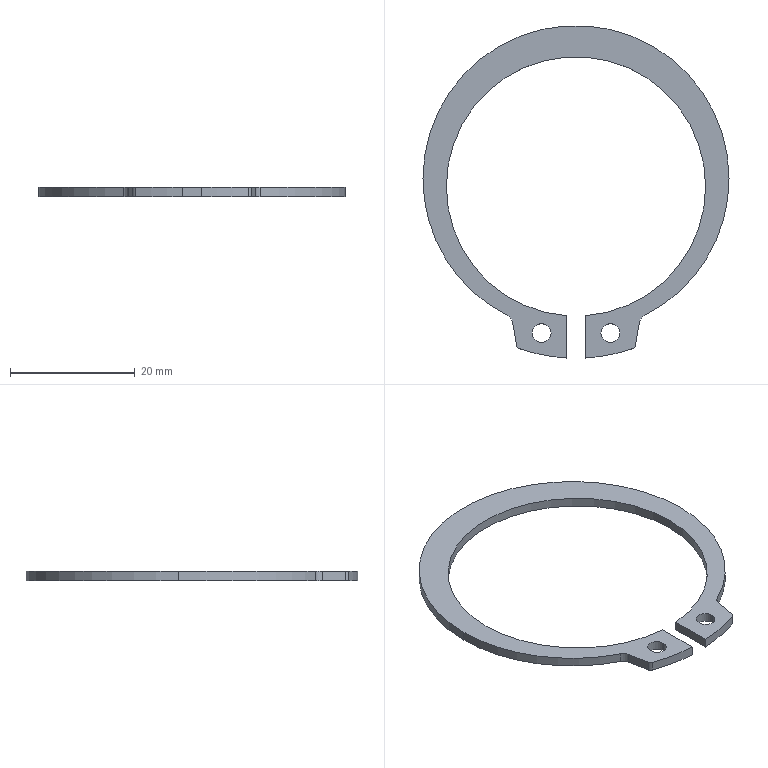Part | SolidWorks | features Extrusion 1 | 1 solid | 22 faces | box 49 x 53.209 x 1.5 mm | volume 876.142 mm3 | cylinder 16 | plane 6 | commonest cylinder face diameters 3 x6 41.5 x3 49 x3 1.4 x2 55 x2
STEP:
#1=CARTESIAN_POINT('',(4.,-24.714,0.75));
#2=VERTEX_POINT('',#1);
#3=CARTESIAN_POINT('',(7.,-24.714,0.75));
#4=VERTEX_POINT('',#3);
#5=CARTESIAN_POINT('',(5.5,-24.714,0.75));
#6=DIRECTION('',(0.,0.,1.));
#7=DIRECTION('',(-1.,0.,0.));
#8=AXIS2_PLACEMENT_3D('',#5,#6,#7);
#9=CIRCLE('',#8,1.5);
#10=EDGE_CURVE('',#2,#4,#9,.T.);
#11=ORIENTED_EDGE('',*,*,#10,.T.);
#12=CARTESIAN_POINT('',(7.,-24.714,-0.75));
#13=VERTEX_POINT('',#12);
#14=CARTESIAN_POINT('',(7.,-24.714,0.75));
#15=DIRECTION('',(0.,0.,-1.));
#16=VECTOR('',#15,1000.);
#17=LINE('',#14,#16);
#18=EDGE_CURVE('',#4,#13,#17,.T.);
#19=ORIENTED_EDGE('',*,*,#18,.T.);
#20=CARTESIAN_POINT('',(4.,-24.714,-0.75));
#21=VERTEX_POINT('',#20);
#22=CARTESIAN_POINT('',(5.5,-24.714,-0.75));
#23=DIRECTION('',(0.,0.,1.));
#24=DIRECTION('',(-1.,0.,0.));
#25=AXIS2_PLACEMENT_3D('',#22,#23,#24);
#26=CIRCLE('',#25,1.5);
#27=EDGE_CURVE('',#21,#13,#26,.T.);
#28=ORIENTED_EDGE('',*,*,#27,.F.);
#29=CARTESIAN_POINT('',(4.,-24.714,0.75));
#30=DIRECTION('',(0.,0.,-1.));
#31=VECTOR('',#30,1000.);
#32=LINE('',#29,#31);
#33=EDGE_CURVE('',#2,#21,#32,.T.);
#34=ORIENTED_EDGE('',*,*,#33,.F.);
#35=EDGE_LOOP('',(#11,#19,#28,#34));
#36=FACE_OUTER_BOUND('',#35,.T.);
#37=CARTESIAN_POINT('',(5.5,-24.714,0.75));
#38=DIRECTION('',(0.,0.,-1.));
#39=DIRECTION('',(-1.,0.,0.));
#40=AXIS2_PLACEMENT_3D('',#37,#38,#39);
#41=CYLINDRICAL_SURFACE('',#40,1.5);
#42=ADVANCED_FACE('',(#36),#41,.F.);
#43=CARTESIAN_POINT('',(-7.,-24.714,0.75));
#44=VERTEX_POINT('',#43);
#45=CARTESIAN_POINT('',(-4.,-24.714,0.75));
#46=VERTEX_POINT('',#45);
#47=CARTESIAN_POINT('',(-5.5,-24.714,0.75));
#48=DIRECTION('',(0.,0.,1.));
#49=DIRECTION('',(1.,0.,0.));
#50=AXIS2_PLACEMENT_3D('',#47,#48,#49);
#51=CIRCLE('',#50,1.5);
#52=EDGE_CURVE('',#44,#46,#51,.T.);
#53=ORIENTED_EDGE('',*,*,#52,.T.);
#54=CARTESIAN_POINT('',(-4.,-24.714,-0.75));
#55=VERTEX_POINT('',#54);
#56=CARTESIAN_POINT('',(-4.,-24.714,0.75));
#57=DIRECTION('',(0.,0.,-1.));
#58=VECTOR('',#57,1000.);
#59=LINE('',#56,#58);
#60=EDGE_CURVE('',#46,#55,#59,.T.);
#61=ORIENTED_EDGE('',*,*,#60,.T.);
#62=CARTESIAN_POINT('',(-7.,-24.714,-0.75));
#63=VERTEX_POINT('',#62);
#64=CARTESIAN_POINT('',(-5.5,-24.714,-0.75));
#65=DIRECTION('',(0.,0.,1.));
#66=DIRECTION('',(1.,0.,0.));
#67=AXIS2_PLACEMENT_3D('',#64,#65,#66);
#68=CIRCLE('',#67,1.5);
#69=EDGE_CURVE('',#63,#55,#68,.T.);
#70=ORIENTED_EDGE('',*,*,#69,.F.);
#71=CARTESIAN_POINT('',(-7.,-24.714,0.75));
#72=DIRECTION('',(0.,0.,-1.));
#73=VECTOR('',#72,1000.);
#74=LINE('',#71,#73);
#75=EDGE_CURVE('',#44,#63,#74,.T.);
#76=ORIENTED_EDGE('',*,*,#75,.F.);
#77=EDGE_LOOP('',(#53,#61,#70,#76));
#78=FACE_OUTER_BOUND('',#77,.T.);
#79=CARTESIAN_POINT('',(-5.5,-24.714,0.75));
#80=DIRECTION('',(0.,0.,-1.));
#81=DIRECTION('',(-1.,0.,0.));
#82=AXIS2_PLACEMENT_3D('',#79,#80,#81);
#83=CYLINDRICAL_SURFACE('',#82,1.5);
#84=ADVANCED_FACE('',(#78),#83,.F.);
#85=CARTESIAN_POINT('',(24.5,0.,0.75));
#86=VERTEX_POINT('',#85);
#87=CARTESIAN_POINT('',(-24.5,0.,0.75));
#88=VERTEX_POINT('',#87);
#89=CARTESIAN_POINT('',(0.,0.,0.75));
#90=DIRECTION('',(0.,0.,1.));
#91=DIRECTION('',(1.,0.,0.));
#92=AXIS2_PLACEMENT_3D('',#89,#90,#91);
#93=CIRCLE('',#92,24.5);
#94=EDGE_CURVE('',#86,#88,#93,.T.);
#95=ORIENTED_EDGE('',*,*,#94,.F.);
#96=CARTESIAN_POINT('',(24.5,0.,-0.75));
#97=VERTEX_POINT('',#96);
#98=CARTESIAN_POINT('',(24.5,0.,0.75));
#99=DIRECTION('',(0.,0.,-1.));
#100=VECTOR('',#99,1000.);
#101=LINE('',#98,#100);
#102=EDGE_CURVE('',#86,#97,#101,.T.);
#103=ORIENTED_EDGE('',*,*,#102,.T.);
#104=CARTESIAN_POINT('',(-24.5,0.,-0.75));
#105=VERTEX_POINT('',#104);
#106=CARTESIAN_POINT('',(0.,0.,-0.75));
#107=DIRECTION('',(0.,0.,1.));
#108=DIRECTION('',(1.,0.,0.));
#109=AXIS2_PLACEMENT_3D('',#106,#107,#108);
#110=CIRCLE('',#109,24.5);
#111=EDGE_CURVE('',#97,#105,#110,.T.);
#112=ORIENTED_EDGE('',*,*,#111,.T.);
#113=CARTESIAN_POINT('',(-24.5,0.,0.75));
#114=DIRECTION('',(0.,0.,-1.));
#115=VECTOR('',#114,1000.);
#116=LINE('',#113,#115);
#117=EDGE_CURVE('',#88,#105,#116,.T.);
#118=ORIENTED_EDGE('',*,*,#117,.F.);
#119=EDGE_LOOP('',(#95,#103,#112,#118));
#120=FACE_OUTER_BOUND('',#119,.T.);
#121=CARTESIAN_POINT('',(0.,0.,0.75));
#122=DIRECTION('',(0.,0.,-1.));
#123=DIRECTION('',(-1.,0.,0.));
#124=AXIS2_PLACEMENT_3D('',#121,#122,#123);
#125=CYLINDRICAL_SURFACE('',#124,24.5);
#126=ADVANCED_FACE('',(#120),#125,.T.);
#127=CARTESIAN_POINT('',(-10.957,-21.914,0.75));
#128=VERTEX_POINT('',#127);
#129=CARTESIAN_POINT('',(0.,0.,0.75));
#130=DIRECTION('',(0.,0.,1.));
#131=DIRECTION('',(1.,0.,0.));
#132=AXIS2_PLACEMENT_3D('',#129,#130,#131);
#133=CIRCLE('',#132,24.5);
#134=EDGE_CURVE('',#88,#128,#133,.T.);
#135=ORIENTED_EDGE('',*,*,#134,.F.);
#136=ORIENTED_EDGE('',*,*,#117,.T.);
#137=CARTESIAN_POINT('',(-10.957,-21.914,-0.75));
#138=VERTEX_POINT('',#137);
#139=CARTESIAN_POINT('',(0.,0.,-0.75));
#140=DIRECTION('',(0.,0.,1.));
#141=DIRECTION('',(1.,0.,0.));
#142=AXIS2_PLACEMENT_3D('',#139,#140,#141);
#143=CIRCLE('',#142,24.5);
#144=EDGE_CURVE('',#105,#138,#143,.T.);
#145=ORIENTED_EDGE('',*,*,#144,.T.);
#146=CARTESIAN_POINT('',(-10.957,-21.914,0.75));
#147=DIRECTION('',(0.,0.,-1.));
#148=VECTOR('',#147,1000.);
#149=LINE('',#146,#148);
#150=EDGE_CURVE('',#128,#138,#149,.T.);
#151=ORIENTED_EDGE('',*,*,#150,.F.);
#152=EDGE_LOOP('',(#135,#136,#145,#151));
#153=FACE_OUTER_BOUND('',#152,.T.);
#154=CARTESIAN_POINT('',(0.,0.,0.75));
#155=DIRECTION('',(0.,0.,-1.));
#156=DIRECTION('',(-1.,0.,0.));
#157=AXIS2_PLACEMENT_3D('',#154,#155,#156);
#158=CYLINDRICAL_SURFACE('',#157,24.5);
#159=ADVANCED_FACE('',(#153),#158,.T.);
#160=CARTESIAN_POINT('',(20.75,-1.25,0.75));
#161=VERTEX_POINT('',#160);
#162=CARTESIAN_POINT('',(1.5,-21.946,0.75));
#163=VERTEX_POINT('',#162);
#164=CARTESIAN_POINT('',(0.,-1.25,0.75));
#165=DIRECTION('',(0.,0.,-1.));
#166=DIRECTION('',(1.,0.,0.));
#167=AXIS2_PLACEMENT_3D('',#164,#165,#166);
#168=CIRCLE('',#167,20.75);
#169=EDGE_CURVE('',#161,#163,#168,.T.);
#170=ORIENTED_EDGE('',*,*,#169,.F.);
#171=CARTESIAN_POINT('',(20.75,-1.25,-0.75));
#172=VERTEX_POINT('',#171);
#173=CARTESIAN_POINT('',(20.75,-1.25,0.75));
#174=DIRECTION('',(0.,0.,-1.));
#175=VECTOR('',#174,1000.);
#176=LINE('',#173,#175);
#177=EDGE_CURVE('',#161,#172,#176,.T.);
#178=ORIENTED_EDGE('',*,*,#177,.T.);
#179=CARTESIAN_POINT('',(1.5,-21.946,-0.75));
#180=VERTEX_POINT('',#179);
#181=CARTESIAN_POINT('',(0.,-1.25,-0.75));
#182=DIRECTION('',(0.,0.,-1.));
#183=DIRECTION('',(1.,0.,0.));
#184=AXIS2_PLACEMENT_3D('',#181,#182,#183);
#185=CIRCLE('',#184,20.75);
#186=EDGE_CURVE('',#172,#180,#185,.T.);
#187=ORIENTED_EDGE('',*,*,#186,.T.);
#188=CARTESIAN_POINT('',(1.5,-21.946,0.75));
#189=DIRECTION('',(0.,0.,-1.));
#190=VECTOR('',#189,1000.);
#191=LINE('',#188,#190);
#192=EDGE_CURVE('',#163,#180,#191,.T.);
#193=ORIENTED_EDGE('',*,*,#192,.F.);
#194=EDGE_LOOP('',(#170,#178,#187,#193));
#195=FACE_OUTER_BOUND('',#194,.T.);
#196=CARTESIAN_POINT('',(0.,-1.25,0.75));
#197=DIRECTION('',(0.,0.,-1.));
#198=DIRECTION('',(-1.,0.,0.));
#199=AXIS2_PLACEMENT_3D('',#196,#197,#198);
#200=CYLINDRICAL_SURFACE('',#199,20.75);
#201=ADVANCED_FACE('',(#195),#200,.F.);
#202=ORIENTED_EDGE('',*,*,#177,.F.);
#203=CARTESIAN_POINT('',(-20.75,-1.25,0.75));
#204=VERTEX_POINT('',#203);
#205=CARTESIAN_POINT('',(0.,-1.25,0.75));
#206=DIRECTION('',(0.,0.,-1.));
#207=DIRECTION('',(1.,0.,0.));
#208=AXIS2_PLACEMENT_3D('',#205,#206,#207);
#209=CIRCLE('',#208,20.75);
#210=EDGE_CURVE('',#204,#161,#209,.T.);
#211=ORIENTED_EDGE('',*,*,#210,.F.);
#212=CARTESIAN_POINT('',(-20.75,-1.25,-0.75));
#213=VERTEX_POINT('',#212);
#214=CARTESIAN_POINT('',(-20.75,-1.25,0.75));
#215=DIRECTION('',(0.,0.,-1.));
#216=VECTOR('',#215,1000.);
#217=LINE('',#214,#216);
#218=EDGE_CURVE('',#204,#213,#217,.T.);
#219=ORIENTED_EDGE('',*,*,#218,.T.);
#220=CARTESIAN_POINT('',(0.,-1.25,-0.75));
#221=DIRECTION('',(0.,0.,-1.));
#222=DIRECTION('',(1.,0.,0.));
#223=AXIS2_PLACEMENT_3D('',#220,#221,#222);
#224=CIRCLE('',#223,20.75);
#225=EDGE_CURVE('',#213,#172,#224,.T.);
#226=ORIENTED_EDGE('',*,*,#225,.T.);
#227=EDGE_LOOP('',(#202,#211,#219,#226));
#228=FACE_OUTER_BOUND('',#227,.T.);
#229=CARTESIAN_POINT('',(0.,-1.25,0.75));
#230=DIRECTION('',(0.,0.,-1.));
#231=DIRECTION('',(-1.,0.,0.));
#232=AXIS2_PLACEMENT_3D('',#229,#230,#231);
#233=CYLINDRICAL_SURFACE('',#232,20.75);
#234=ADVANCED_FACE('',(#228),#233,.F.);
#235=ORIENTED_EDGE('',*,*,#52,.F.);
#236=CARTESIAN_POINT('',(-5.5,-24.714,0.75));
#237=DIRECTION('',(0.,0.,1.));
#238=DIRECTION('',(1.,0.,0.));
#239=AXIS2_PLACEMENT_3D('',#236,#237,#238);
#240=CIRCLE('',#239,1.5);
#241=EDGE_CURVE('',#46,#44,#240,.T.);
#242=ORIENTED_EDGE('',*,*,#241,.F.);
#243=EDGE_LOOP('',(#235,#242));
#244=FACE_BOUND('',#243,.T.);
#245=CARTESIAN_POINT('',(-10.15,-22.995,0.75));
#246=VERTEX_POINT('',#245);
#247=CARTESIAN_POINT('',(-11.627,-23.255,0.75));
#248=DIRECTION('',(0.,0.,-1.));
#249=DIRECTION('',(1.,0.,0.));
#250=AXIS2_PLACEMENT_3D('',#247,#248,#249);
#251=CIRCLE('',#250,1.5);
#252=EDGE_CURVE('',#128,#246,#251,.T.);
#253=ORIENTED_EDGE('',*,*,#252,.T.);
#254=CARTESIAN_POINT('',(-9.5,-26.682,0.75));
#255=VERTEX_POINT('',#254);
#256=CARTESIAN_POINT('',(-10.15,-22.995,0.75));
#257=DIRECTION('',(0.1736,-0.9848,0.));
#258=VECTOR('',#257,1000.);
#259=LINE('',#256,#258);
#260=EDGE_CURVE('',#246,#255,#259,.T.);
#261=ORIENTED_EDGE('',*,*,#260,.T.);
#262=CARTESIAN_POINT('',(-9.041,-27.221,0.75));
#263=VERTEX_POINT('',#262);
#264=CARTESIAN_POINT('',(-8.811,-26.56,0.75));
#265=DIRECTION('',(0.,0.,1.));
#266=DIRECTION('',(-1.,0.,0.));
#267=AXIS2_PLACEMENT_3D('',#264,#265,#266);
#268=CIRCLE('',#267,0.7);
#269=EDGE_CURVE('',#255,#263,#268,.T.);
#270=ORIENTED_EDGE('',*,*,#269,.T.);
#271=CARTESIAN_POINT('',(-1.5,-28.709,0.75));
#272=VERTEX_POINT('',#271);
#273=CARTESIAN_POINT('',(0.,-1.25,0.75));
#274=DIRECTION('',(0.,0.,1.));
#275=DIRECTION('',(-1.,0.,0.));
#276=AXIS2_PLACEMENT_3D('',#273,#274,#275);
#277=CIRCLE('',#276,27.5);
#278=EDGE_CURVE('',#263,#272,#277,.T.);
#279=ORIENTED_EDGE('',*,*,#278,.T.);
#280=CARTESIAN_POINT('',(-1.5,-21.946,0.75));
#281=VERTEX_POINT('',#280);
#282=CARTESIAN_POINT('',(-1.5,-21.946,0.75));
#283=DIRECTION('',(0.,1.,0.));
#284=VECTOR('',#283,1000.);
#285=LINE('',#282,#284);
#286=EDGE_CURVE('',#272,#281,#285,.T.);
#287=ORIENTED_EDGE('',*,*,#286,.T.);
#288=CARTESIAN_POINT('',(0.,-1.25,0.75));
#289=DIRECTION('',(0.,0.,-1.));
#290=DIRECTION('',(1.,0.,0.));
#291=AXIS2_PLACEMENT_3D('',#288,#289,#290);
#292=CIRCLE('',#291,20.75);
#293=EDGE_CURVE('',#281,#204,#292,.T.);
#294=ORIENTED_EDGE('',*,*,#293,.T.);
#295=ORIENTED_EDGE('',*,*,#210,.T.);
#296=ORIENTED_EDGE('',*,*,#169,.T.);
#297=CARTESIAN_POINT('',(1.5,-28.709,0.75));
#298=VERTEX_POINT('',#297);
#299=CARTESIAN_POINT('',(1.5,-21.946,0.75));
#300=DIRECTION('',(0.,-1.,0.));
#301=VECTOR('',#300,1000.);
#302=LINE('',#299,#301);
#303=EDGE_CURVE('',#163,#298,#302,.T.);
#304=ORIENTED_EDGE('',*,*,#303,.T.);
#305=CARTESIAN_POINT('',(9.041,-27.221,0.75));
#306=VERTEX_POINT('',#305);
#307=CARTESIAN_POINT('',(0.,-1.25,0.75));
#308=DIRECTION('',(0.,0.,1.));
#309=DIRECTION('',(1.,0.,0.));
#310=AXIS2_PLACEMENT_3D('',#307,#308,#309);
#311=CIRCLE('',#310,27.5);
#312=EDGE_CURVE('',#298,#306,#311,.T.);
#313=ORIENTED_EDGE('',*,*,#312,.T.);
#314=CARTESIAN_POINT('',(9.5,-26.682,0.75));
#315=VERTEX_POINT('',#314);
#316=CARTESIAN_POINT('',(8.811,-26.56,0.75));
#317=DIRECTION('',(0.,0.,1.));
#318=DIRECTION('',(1.,0.,0.));
#319=AXIS2_PLACEMENT_3D('',#316,#317,#318);
#320=CIRCLE('',#319,0.7);
#321=EDGE_CURVE('',#306,#315,#320,.T.);
#322=ORIENTED_EDGE('',*,*,#321,.T.);
#323=CARTESIAN_POINT('',(10.15,-22.995,0.75));
#324=VERTEX_POINT('',#323);
#325=CARTESIAN_POINT('',(10.15,-22.995,0.75));
#326=DIRECTION('',(0.1736,0.9848,0.));
#327=VECTOR('',#326,1000.);
#328=LINE('',#325,#327);
#329=EDGE_CURVE('',#315,#324,#328,.T.);
#330=ORIENTED_EDGE('',*,*,#329,.T.);
#331=CARTESIAN_POINT('',(10.957,-21.914,0.75));
#332=VERTEX_POINT('',#331);
#333=CARTESIAN_POINT('',(11.627,-23.255,0.75));
#334=DIRECTION('',(0.,0.,-1.));
#335=DIRECTION('',(-1.,0.,0.));
#336=AXIS2_PLACEMENT_3D('',#333,#334,#335);
#337=CIRCLE('',#336,1.5);
#338=EDGE_CURVE('',#324,#332,#337,.T.);
#339=ORIENTED_EDGE('',*,*,#338,.T.);
#340=CARTESIAN_POINT('',(0.,0.,0.75));
#341=DIRECTION('',(0.,0.,1.));
#342=DIRECTION('',(1.,0.,0.));
#343=AXIS2_PLACEMENT_3D('',#340,#341,#342);
#344=CIRCLE('',#343,24.5);
#345=EDGE_CURVE('',#332,#86,#344,.T.);
#346=ORIENTED_EDGE('',*,*,#345,.T.);
#347=ORIENTED_EDGE('',*,*,#94,.T.);
#348=ORIENTED_EDGE('',*,*,#134,.T.);
#349=EDGE_LOOP('',(#253,#261,#270,#279,#287,#294,#295,#296,#304,#313,#322,#330,#339,#346,#347,#348));
#350=FACE_OUTER_BOUND('',#349,.T.);
#351=ORIENTED_EDGE('',*,*,#10,.F.);
#352=CARTESIAN_POINT('',(5.5,-24.714,0.75));
#353=DIRECTION('',(0.,0.,1.));
#354=DIRECTION('',(-1.,0.,0.));
#355=AXIS2_PLACEMENT_3D('',#352,#353,#354);
#356=CIRCLE('',#355,1.5);
#357=EDGE_CURVE('',#4,#2,#356,.T.);
#358=ORIENTED_EDGE('',*,*,#357,.F.);
#359=EDGE_LOOP('',(#351,#358));
#360=FACE_BOUND('',#359,.T.);
#361=CARTESIAN_POINT('',(-11.627,-23.255,0.75));
#362=DIRECTION('',(0.,0.,1.));
#363=DIRECTION('',(1.,0.,0.));
#364=AXIS2_PLACEMENT_3D('',#361,#362,#363);
#365=PLANE('',#364);
#366=ADVANCED_FACE('',(#244,#350,#360),#365,.T.);
#367=ORIENTED_EDGE('',*,*,#150,.T.);
#368=CARTESIAN_POINT('',(-10.15,-22.995,-0.75));
#369=VERTEX_POINT('',#368);
#370=CARTESIAN_POINT('',(-11.627,-23.255,-0.75));
#371=DIRECTION('',(0.,0.,-1.));
#372=DIRECTION('',(1.,0.,0.));
#373=AXIS2_PLACEMENT_3D('',#370,#371,#372);
#374=CIRCLE('',#373,1.5);
#375=EDGE_CURVE('',#138,#369,#374,.T.);
#376=ORIENTED_EDGE('',*,*,#375,.T.);
#377=CARTESIAN_POINT('',(-10.15,-22.995,0.75));
#378=DIRECTION('',(0.,0.,-1.));
#379=VECTOR('',#378,1000.);
#380=LINE('',#377,#379);
#381=EDGE_CURVE('',#246,#369,#380,.T.);
#382=ORIENTED_EDGE('',*,*,#381,.F.);
#383=ORIENTED_EDGE('',*,*,#252,.F.);
#384=EDGE_LOOP('',(#367,#376,#382,#383));
#385=FACE_OUTER_BOUND('',#384,.T.);
#386=CARTESIAN_POINT('',(-11.627,-23.255,0.75));
#387=DIRECTION('',(0.,0.,-1.));
#388=DIRECTION('',(-1.,0.,0.));
#389=AXIS2_PLACEMENT_3D('',#386,#387,#388);
#390=CYLINDRICAL_SURFACE('',#389,1.5);
#391=ADVANCED_FACE('',(#385),#390,.F.);
#392=ORIENTED_EDGE('',*,*,#381,.T.);
#393=CARTESIAN_POINT('',(-9.5,-26.682,-0.75));
#394=VERTEX_POINT('',#393);
#395=CARTESIAN_POINT('',(-10.15,-22.995,-0.75));
#396=DIRECTION('',(0.1736,-0.9848,0.));
#397=VECTOR('',#396,1000.);
#398=LINE('',#395,#397);
#399=EDGE_CURVE('',#369,#394,#398,.T.);
#400=ORIENTED_EDGE('',*,*,#399,.T.);
#401=CARTESIAN_POINT('',(-9.5,-26.682,0.75));
#402=DIRECTION('',(0.,0.,-1.));
#403=VECTOR('',#402,1000.);
#404=LINE('',#401,#403);
#405=EDGE_CURVE('',#255,#394,#404,.T.);
#406=ORIENTED_EDGE('',*,*,#405,.F.);
#407=ORIENTED_EDGE('',*,*,#260,.F.);
#408=EDGE_LOOP('',(#392,#400,#406,#407));
#409=FACE_OUTER_BOUND('',#408,.T.);
#410=CARTESIAN_POINT('',(-10.15,-22.995,0.75));
#411=DIRECTION('',(0.9848,0.1736,0.));
#412=DIRECTION('',(-0.1736,0.9848,0.));
#413=AXIS2_PLACEMENT_3D('',#410,#411,#412);
#414=PLANE('',#413);
#415=ADVANCED_FACE('',(#409),#414,.F.);
#416=ORIENTED_EDGE('',*,*,#405,.T.);
#417=CARTESIAN_POINT('',(-9.041,-27.221,-0.75));
#418=VERTEX_POINT('',#417);
#419=CARTESIAN_POINT('',(-8.811,-26.56,-0.75));
#420=DIRECTION('',(0.,0.,1.));
#421=DIRECTION('',(-1.,0.,0.));
#422=AXIS2_PLACEMENT_3D('',#419,#420,#421);
#423=CIRCLE('',#422,0.7);
#424=EDGE_CURVE('',#394,#418,#423,.T.);
#425=ORIENTED_EDGE('',*,*,#424,.T.);
#426=CARTESIAN_POINT('',(-9.041,-27.221,0.75));
#427=DIRECTION('',(0.,0.,-1.));
#428=VECTOR('',#427,1000.);
#429=LINE('',#426,#428);
#430=EDGE_CURVE('',#263,#418,#429,.T.);
#431=ORIENTED_EDGE('',*,*,#430,.F.);
#432=ORIENTED_EDGE('',*,*,#269,.F.);
#433=EDGE_LOOP('',(#416,#425,#431,#432));
#434=FACE_OUTER_BOUND('',#433,.T.);
#435=CARTESIAN_POINT('',(-8.811,-26.56,0.75));
#436=DIRECTION('',(0.,0.,-1.));
#437=DIRECTION('',(-1.,0.,0.));
#438=AXIS2_PLACEMENT_3D('',#435,#436,#437);
#439=CYLINDRICAL_SURFACE('',#438,0.7);
#440=ADVANCED_FACE('',(#434),#439,.T.);
#441=ORIENTED_EDGE('',*,*,#430,.T.);
#442=CARTESIAN_POINT('',(-1.5,-28.709,-0.75));
#443=VERTEX_POINT('',#442);
#444=CARTESIAN_POINT('',(0.,-1.25,-0.75));
#445=DIRECTION('',(0.,0.,1.));
#446=DIRECTION('',(-1.,0.,0.));
#447=AXIS2_PLACEMENT_3D('',#444,#445,#446);
#448=CIRCLE('',#447,27.5);
#449=EDGE_CURVE('',#418,#443,#448,.T.);
#450=ORIENTED_EDGE('',*,*,#449,.T.);
#451=CARTESIAN_POINT('',(-1.5,-28.709,0.75));
#452=DIRECTION('',(0.,0.,-1.));
#453=VECTOR('',#452,1000.);
#454=LINE('',#451,#453);
#455=EDGE_CURVE('',#272,#443,#454,.T.);
#456=ORIENTED_EDGE('',*,*,#455,.F.);
#457=ORIENTED_EDGE('',*,*,#278,.F.);
#458=EDGE_LOOP('',(#441,#450,#456,#457));
#459=FACE_OUTER_BOUND('',#458,.T.);
#460=CARTESIAN_POINT('',(0.,-1.25,0.75));
#461=DIRECTION('',(0.,0.,-1.));
#462=DIRECTION('',(-1.,0.,0.));
#463=AXIS2_PLACEMENT_3D('',#460,#461,#462);
#464=CYLINDRICAL_SURFACE('',#463,27.5);
#465=ADVANCED_FACE('',(#459),#464,.T.);
#466=ORIENTED_EDGE('',*,*,#455,.T.);
#467=CARTESIAN_POINT('',(-1.5,-21.946,-0.75));
#468=VERTEX_POINT('',#467);
#469=CARTESIAN_POINT('',(-1.5,-21.946,-0.75));
#470=DIRECTION('',(0.,1.,0.));
#471=VECTOR('',#470,1000.);
#472=LINE('',#469,#471);
#473=EDGE_CURVE('',#443,#468,#472,.T.);
#474=ORIENTED_EDGE('',*,*,#473,.T.);
#475=CARTESIAN_POINT('',(-1.5,-21.946,0.75));
#476=DIRECTION('',(0.,0.,-1.));
#477=VECTOR('',#476,1000.);
#478=LINE('',#475,#477);
#479=EDGE_CURVE('',#281,#468,#478,.T.);
#480=ORIENTED_EDGE('',*,*,#479,.F.);
#481=ORIENTED_EDGE('',*,*,#286,.F.);
#482=EDGE_LOOP('',(#466,#474,#480,#481));
#483=FACE_OUTER_BOUND('',#482,.T.);
#484=CARTESIAN_POINT('',(-1.5,-21.946,0.75));
#485=DIRECTION('',(-1.,0.,0.));
#486=DIRECTION('',(0.,-1.,0.));
#487=AXIS2_PLACEMENT_3D('',#484,#485,#486);
#488=PLANE('',#487);
#489=ADVANCED_FACE('',(#483),#488,.F.);
#490=ORIENTED_EDGE('',*,*,#218,.F.);
#491=ORIENTED_EDGE('',*,*,#293,.F.);
#492=ORIENTED_EDGE('',*,*,#479,.T.);
#493=CARTESIAN_POINT('',(0.,-1.25,-0.75));
#494=DIRECTION('',(0.,0.,-1.));
#495=DIRECTION('',(1.,0.,0.));
#496=AXIS2_PLACEMENT_3D('',#493,#494,#495);
#497=CIRCLE('',#496,20.75);
#498=EDGE_CURVE('',#468,#213,#497,.T.);
#499=ORIENTED_EDGE('',*,*,#498,.T.);
#500=EDGE_LOOP('',(#490,#491,#492,#499));
#501=FACE_OUTER_BOUND('',#500,.T.);
#502=CARTESIAN_POINT('',(0.,-1.25,0.75));
#503=DIRECTION('',(0.,0.,-1.));
#504=DIRECTION('',(-1.,0.,0.));
#505=AXIS2_PLACEMENT_3D('',#502,#503,#504);
#506=CYLINDRICAL_SURFACE('',#505,20.75);
#507=ADVANCED_FACE('',(#501),#506,.F.);
#508=ORIENTED_EDGE('',*,*,#192,.T.);
#509=CARTESIAN_POINT('',(1.5,-28.709,-0.75));
#510=VERTEX_POINT('',#509);
#511=CARTESIAN_POINT('',(1.5,-21.946,-0.75));
#512=DIRECTION('',(0.,-1.,0.));
#513=VECTOR('',#512,1000.);
#514=LINE('',#511,#513);
#515=EDGE_CURVE('',#180,#510,#514,.T.);
#516=ORIENTED_EDGE('',*,*,#515,.T.);
#517=CARTESIAN_POINT('',(1.5,-28.709,0.75));
#518=DIRECTION('',(0.,0.,-1.));
#519=VECTOR('',#518,1000.);
#520=LINE('',#517,#519);
#521=EDGE_CURVE('',#298,#510,#520,.T.);
#522=ORIENTED_EDGE('',*,*,#521,.F.);
#523=ORIENTED_EDGE('',*,*,#303,.F.);
#524=EDGE_LOOP('',(#508,#516,#522,#523));
#525=FACE_OUTER_BOUND('',#524,.T.);
#526=CARTESIAN_POINT('',(1.5,-21.946,0.75));
#527=DIRECTION('',(1.,0.,0.));
#528=DIRECTION('',(0.,1.,0.));
#529=AXIS2_PLACEMENT_3D('',#526,#527,#528);
#530=PLANE('',#529);
#531=ADVANCED_FACE('',(#525),#530,.F.);
#532=ORIENTED_EDGE('',*,*,#521,.T.);
#533=CARTESIAN_POINT('',(9.041,-27.221,-0.75));
#534=VERTEX_POINT('',#533);
#535=CARTESIAN_POINT('',(0.,-1.25,-0.75));
#536=DIRECTION('',(0.,0.,1.));
#537=DIRECTION('',(1.,0.,0.));
#538=AXIS2_PLACEMENT_3D('',#535,#536,#537);
#539=CIRCLE('',#538,27.5);
#540=EDGE_CURVE('',#510,#534,#539,.T.);
#541=ORIENTED_EDGE('',*,*,#540,.T.);
#542=CARTESIAN_POINT('',(9.041,-27.221,0.75));
#543=DIRECTION('',(0.,0.,-1.));
#544=VECTOR('',#543,1000.);
#545=LINE('',#542,#544);
#546=EDGE_CURVE('',#306,#534,#545,.T.);
#547=ORIENTED_EDGE('',*,*,#546,.F.);
#548=ORIENTED_EDGE('',*,*,#312,.F.);
#549=EDGE_LOOP('',(#532,#541,#547,#548));
#550=FACE_OUTER_BOUND('',#549,.T.);
#551=CARTESIAN_POINT('',(0.,-1.25,0.75));
#552=DIRECTION('',(0.,0.,-1.));
#553=DIRECTION('',(-1.,0.,0.));
#554=AXIS2_PLACEMENT_3D('',#551,#552,#553);
#555=CYLINDRICAL_SURFACE('',#554,27.5);
#556=ADVANCED_FACE('',(#550),#555,.T.);
#557=ORIENTED_EDGE('',*,*,#546,.T.);
#558=CARTESIAN_POINT('',(9.5,-26.682,-0.75));
#559=VERTEX_POINT('',#558);
#560=CARTESIAN_POINT('',(8.811,-26.56,-0.75));
#561=DIRECTION('',(0.,0.,1.));
#562=DIRECTION('',(1.,0.,0.));
#563=AXIS2_PLACEMENT_3D('',#560,#561,#562);
#564=CIRCLE('',#563,0.7);
#565=EDGE_CURVE('',#534,#559,#564,.T.);
#566=ORIENTED_EDGE('',*,*,#565,.T.);
#567=CARTESIAN_POINT('',(9.5,-26.682,0.75));
#568=DIRECTION('',(0.,0.,-1.));
#569=VECTOR('',#568,1000.);
#570=LINE('',#567,#569);
#571=EDGE_CURVE('',#315,#559,#570,.T.);
#572=ORIENTED_EDGE('',*,*,#571,.F.);
#573=ORIENTED_EDGE('',*,*,#321,.F.);
#574=EDGE_LOOP('',(#557,#566,#572,#573));
#575=FACE_OUTER_BOUND('',#574,.T.);
#576=CARTESIAN_POINT('',(8.811,-26.56,0.75));
#577=DIRECTION('',(0.,0.,-1.));
#578=DIRECTION('',(-1.,0.,0.));
#579=AXIS2_PLACEMENT_3D('',#576,#577,#578);
#580=CYLINDRICAL_SURFACE('',#579,0.7);
#581=ADVANCED_FACE('',(#575),#580,.T.);
#582=ORIENTED_EDGE('',*,*,#571,.T.);
#583=CARTESIAN_POINT('',(10.15,-22.995,-0.75));
#584=VERTEX_POINT('',#583);
#585=CARTESIAN_POINT('',(10.15,-22.995,-0.75));
#586=DIRECTION('',(0.1736,0.9848,0.));
#587=VECTOR('',#586,1000.);
#588=LINE('',#585,#587);
#589=EDGE_CURVE('',#559,#584,#588,.T.);
#590=ORIENTED_EDGE('',*,*,#589,.T.);
#591=CARTESIAN_POINT('',(10.15,-22.995,0.75));
#592=DIRECTION('',(0.,0.,-1.));
#593=VECTOR('',#592,1000.);
#594=LINE('',#591,#593);
#595=EDGE_CURVE('',#324,#584,#594,.T.);
#596=ORIENTED_EDGE('',*,*,#595,.F.);
#597=ORIENTED_EDGE('',*,*,#329,.F.);
#598=EDGE_LOOP('',(#582,#590,#596,#597));
#599=FACE_OUTER_BOUND('',#598,.T.);
#600=CARTESIAN_POINT('',(10.15,-22.995,0.75));
#601=DIRECTION('',(-0.9848,0.1736,0.));
#602=DIRECTION('',(-0.1736,-0.9848,0.));
#603=AXIS2_PLACEMENT_3D('',#600,#601,#602);
#604=PLANE('',#603);
#605=ADVANCED_FACE('',(#599),#604,.F.);
#606=ORIENTED_EDGE('',*,*,#595,.T.);
#607=CARTESIAN_POINT('',(10.957,-21.914,-0.75));
#608=VERTEX_POINT('',#607);
#609=CARTESIAN_POINT('',(11.627,-23.255,-0.75));
#610=DIRECTION('',(0.,0.,-1.));
#611=DIRECTION('',(-1.,0.,0.));
#612=AXIS2_PLACEMENT_3D('',#609,#610,#611);
#613=CIRCLE('',#612,1.5);
#614=EDGE_CURVE('',#584,#608,#613,.T.);
#615=ORIENTED_EDGE('',*,*,#614,.T.);
#616=CARTESIAN_POINT('',(10.957,-21.914,0.75));
#617=DIRECTION('',(0.,0.,-1.));
#618=VECTOR('',#617,1000.);
#619=LINE('',#616,#618);
#620=EDGE_CURVE('',#332,#608,#619,.T.);
#621=ORIENTED_EDGE('',*,*,#620,.F.);
#622=ORIENTED_EDGE('',*,*,#338,.F.);
#623=EDGE_LOOP('',(#606,#615,#621,#622));
#624=FACE_OUTER_BOUND('',#623,.T.);
#625=CARTESIAN_POINT('',(11.627,-23.255,0.75));
#626=DIRECTION('',(0.,0.,-1.));
#627=DIRECTION('',(-1.,0.,0.));
#628=AXIS2_PLACEMENT_3D('',#625,#626,#627);
#629=CYLINDRICAL_SURFACE('',#628,1.5);
#630=ADVANCED_FACE('',(#624),#629,.F.);
#631=ORIENTED_EDGE('',*,*,#102,.F.);
#632=ORIENTED_EDGE('',*,*,#345,.F.);
#633=ORIENTED_EDGE('',*,*,#620,.T.);
#634=CARTESIAN_POINT('',(0.,0.,-0.75));
#635=DIRECTION('',(0.,0.,1.));
#636=DIRECTION('',(1.,0.,0.));
#637=AXIS2_PLACEMENT_3D('',#634,#635,#636);
#638=CIRCLE('',#637,24.5);
#639=EDGE_CURVE('',#608,#97,#638,.T.);
#640=ORIENTED_EDGE('',*,*,#639,.T.);
#641=EDGE_LOOP('',(#631,#632,#633,#640));
#642=FACE_OUTER_BOUND('',#641,.T.);
#643=CARTESIAN_POINT('',(0.,0.,0.75));
#644=DIRECTION('',(0.,0.,-1.));
#645=DIRECTION('',(-1.,0.,0.));
#646=AXIS2_PLACEMENT_3D('',#643,#644,#645);
#647=CYLINDRICAL_SURFACE('',#646,24.5);
#648=ADVANCED_FACE('',(#642),#647,.T.);
#649=ORIENTED_EDGE('',*,*,#60,.F.);
#650=ORIENTED_EDGE('',*,*,#241,.T.);
#651=ORIENTED_EDGE('',*,*,#75,.T.);
#652=CARTESIAN_POINT('',(-5.5,-24.714,-0.75));
#653=DIRECTION('',(0.,0.,1.));
#654=DIRECTION('',(1.,0.,0.));
#655=AXIS2_PLACEMENT_3D('',#652,#653,#654);
#656=CIRCLE('',#655,1.5);
#657=EDGE_CURVE('',#55,#63,#656,.T.);
#658=ORIENTED_EDGE('',*,*,#657,.F.);
#659=EDGE_LOOP('',(#649,#650,#651,#658));
#660=FACE_OUTER_BOUND('',#659,.T.);
#661=CARTESIAN_POINT('',(-5.5,-24.714,0.75));
#662=DIRECTION('',(0.,0.,-1.));
#663=DIRECTION('',(-1.,0.,0.));
#664=AXIS2_PLACEMENT_3D('',#661,#662,#663);
#665=CYLINDRICAL_SURFACE('',#664,1.5);
#666=ADVANCED_FACE('',(#660),#665,.F.);
#667=ORIENTED_EDGE('',*,*,#18,.F.);
#668=ORIENTED_EDGE('',*,*,#357,.T.);
#669=ORIENTED_EDGE('',*,*,#33,.T.);
#670=CARTESIAN_POINT('',(5.5,-24.714,-0.75));
#671=DIRECTION('',(0.,0.,1.));
#672=DIRECTION('',(-1.,0.,0.));
#673=AXIS2_PLACEMENT_3D('',#670,#671,#672);
#674=CIRCLE('',#673,1.5);
#675=EDGE_CURVE('',#13,#21,#674,.T.);
#676=ORIENTED_EDGE('',*,*,#675,.F.);
#677=EDGE_LOOP('',(#667,#668,#669,#676));
#678=FACE_OUTER_BOUND('',#677,.T.);
#679=CARTESIAN_POINT('',(5.5,-24.714,0.75));
#680=DIRECTION('',(0.,0.,-1.));
#681=DIRECTION('',(-1.,0.,0.));
#682=AXIS2_PLACEMENT_3D('',#679,#680,#681);
#683=CYLINDRICAL_SURFACE('',#682,1.5);
#684=ADVANCED_FACE('',(#678),#683,.F.);
#685=ORIENTED_EDGE('',*,*,#27,.T.);
#686=ORIENTED_EDGE('',*,*,#675,.T.);
#687=EDGE_LOOP('',(#685,#686));
#688=FACE_BOUND('',#687,.T.);
#689=ORIENTED_EDGE('',*,*,#69,.T.);
#690=ORIENTED_EDGE('',*,*,#657,.T.);
#691=EDGE_LOOP('',(#689,#690));
#692=FACE_BOUND('',#691,.T.);
#693=ORIENTED_EDGE('',*,*,#375,.F.);
#694=ORIENTED_EDGE('',*,*,#144,.F.);
#695=ORIENTED_EDGE('',*,*,#111,.F.);
#696=ORIENTED_EDGE('',*,*,#639,.F.);
#697=ORIENTED_EDGE('',*,*,#614,.F.);
#698=ORIENTED_EDGE('',*,*,#589,.F.);
#699=ORIENTED_EDGE('',*,*,#565,.F.);
#700=ORIENTED_EDGE('',*,*,#540,.F.);
#701=ORIENTED_EDGE('',*,*,#515,.F.);
#702=ORIENTED_EDGE('',*,*,#186,.F.);
#703=ORIENTED_EDGE('',*,*,#225,.F.);
#704=ORIENTED_EDGE('',*,*,#498,.F.);
#705=ORIENTED_EDGE('',*,*,#473,.F.);
#706=ORIENTED_EDGE('',*,*,#449,.F.);
#707=ORIENTED_EDGE('',*,*,#424,.F.);
#708=ORIENTED_EDGE('',*,*,#399,.F.);
#709=EDGE_LOOP('',(#693,#694,#695,#696,#697,#698,#699,#700,#701,#702,#703,#704,#705,#706,#707,#708));
#710=FACE_OUTER_BOUND('',#709,.T.);
#711=CARTESIAN_POINT('',(-11.627,-23.255,-0.75));
#712=DIRECTION('',(0.,0.,1.));
#713=DIRECTION('',(1.,0.,0.));
#714=AXIS2_PLACEMENT_3D('',#711,#712,#713);
#715=PLANE('',#714);
#716=ADVANCED_FACE('',(#688,#692,#710),#715,.F.);
#717=CLOSED_SHELL('',(#42,#84,#126,#159,#201,#234,#366,#391,#415,#440,#465,#489,#507,#531,#556,#581,#605,#630,#648,#666,#684,#716));
#718=MANIFOLD_SOLID_BREP('',#717);
#719=CARTESIAN_POINT('',(0.,0.,0.));
#720=DIRECTION('',(0.,0.,1.));
#721=DIRECTION('',(1.,0.,0.));
#722=AXIS2_PLACEMENT_3D('',#719,#720,#721);
#723=(LENGTH_UNIT()NAMED_UNIT(*)SI_UNIT(.MILLI.,.METRE.));
#724=UNCERTAINTY_MEASURE_WITH_UNIT(LENGTH_MEASURE(0.00001),#723,'','');
#725=(NAMED_UNIT(*)PLANE_ANGLE_UNIT()SI_UNIT($,.RADIAN.));
#726=(NAMED_UNIT(*)SI_UNIT($,.STERADIAN.)SOLID_ANGLE_UNIT());
#727=(GEOMETRIC_REPRESENTATION_CONTEXT(3)GLOBAL_UNCERTAINTY_ASSIGNED_CONTEXT((#724))GLOBAL_UNIT_ASSIGNED_CONTEXT((#723,#725,#726))REPRESENTATION_CONTEXT('',''));
#728=ADVANCED_BREP_SHAPE_REPRESENTATION('',(#718,#722),#727);